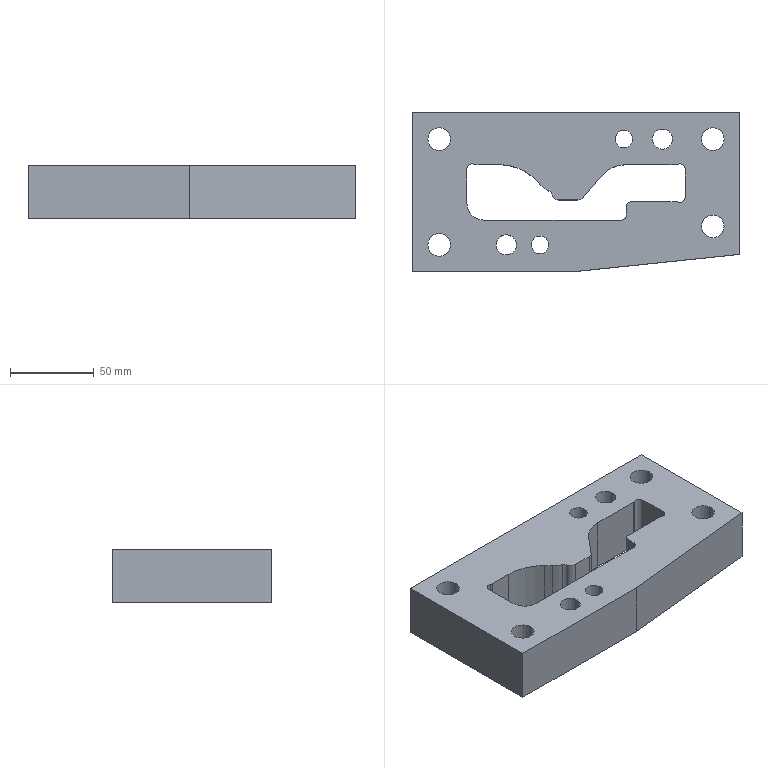Part | STEP file | lll_id254_x_t | 1 solid | 48 faces | box 195 x 95 x 32 mm | volume 434592 mm3 | cylinder 27 | plane 21 | commonest cylinder face diameters 6 x8 13.509 x4 20.008 x4 8 x3 10.505 x2 12 x2
STEP:
#1=CARTESIAN_POINT('',(479.5,-12.921,92.5));
#2=VERTEX_POINT('',#1);
#3=CARTESIAN_POINT('',(380.426,-23.25,92.5));
#4=VERTEX_POINT('',#3);
#5=CARTESIAN_POINT('',(386.882,-22.577,92.5));
#6=DIRECTION('',(-0.9946,-0.1037,0.));
#7=VECTOR('',#6,1.);
#8=LINE('',#5,#7);
#9=EDGE_CURVE('',#2,#4,#8,.T.);
#10=ORIENTED_EDGE('',*,*,#9,.F.);
#11=CARTESIAN_POINT('',(479.5,71.75,92.5));
#12=VERTEX_POINT('',#11);
#13=CARTESIAN_POINT('',(479.5,24.25,92.5));
#14=DIRECTION('',(0.,-1.,0.));
#15=VECTOR('',#14,1.);
#16=LINE('',#13,#15);
#17=EDGE_CURVE('',#12,#2,#16,.T.);
#18=ORIENTED_EDGE('',*,*,#17,.F.);
#19=CARTESIAN_POINT('',(284.5,71.75,92.5));
#20=VERTEX_POINT('',#19);
#21=CARTESIAN_POINT('',(382.,71.75,92.5));
#22=DIRECTION('',(1.,0.,0.));
#23=VECTOR('',#22,1.);
#24=LINE('',#21,#23);
#25=EDGE_CURVE('',#20,#12,#24,.T.);
#26=ORIENTED_EDGE('',*,*,#25,.F.);
#27=CARTESIAN_POINT('',(284.5,-23.25,92.5));
#28=VERTEX_POINT('',#27);
#29=CARTESIAN_POINT('',(284.5,24.25,92.5));
#30=DIRECTION('',(0.,1.,0.));
#31=VECTOR('',#30,1.);
#32=LINE('',#29,#31);
#33=EDGE_CURVE('',#28,#20,#32,.T.);
#34=ORIENTED_EDGE('',*,*,#33,.F.);
#35=CARTESIAN_POINT('',(382.,-23.25,92.5));
#36=DIRECTION('',(-1.,0.,0.));
#37=VECTOR('',#36,1.);
#38=LINE('',#35,#37);
#39=EDGE_CURVE('',#4,#28,#38,.T.);
#40=ORIENTED_EDGE('',*,*,#39,.F.);
#41=EDGE_LOOP('',(#10,#18,#26,#34,#40));
#42=FACE_BOUND('',#41,.T.);
#43=CARTESIAN_POINT('',(334.5,-7.25,92.5));
#44=VERTEX_POINT('',#43);
#45=CARTESIAN_POINT('',(340.5,-7.25,92.5));
#46=DIRECTION('',(0.,0.,1.));
#47=DIRECTION('',(-1.,0.,0.));
#48=AXIS2_PLACEMENT_3D('',#45,#46,#47);
#49=CIRCLE('',#48,6.);
#50=EDGE_CURVE('',#44,#44,#49,.T.);
#51=ORIENTED_EDGE('',*,*,#50,.F.);
#52=EDGE_LOOP('',(#51));
#53=FACE_BOUND('',#52,.T.);
#54=CARTESIAN_POINT('',(427.5,55.75,92.5));
#55=VERTEX_POINT('',#54);
#56=CARTESIAN_POINT('',(433.5,55.75,92.5));
#57=DIRECTION('',(0.,0.,1.));
#58=DIRECTION('',(-1.,0.,0.));
#59=AXIS2_PLACEMENT_3D('',#56,#57,#58);
#60=CIRCLE('',#59,6.);
#61=EDGE_CURVE('',#55,#55,#60,.T.);
#62=ORIENTED_EDGE('',*,*,#61,.F.);
#63=EDGE_LOOP('',(#62));
#64=FACE_BOUND('',#63,.T.);
#65=CARTESIAN_POINT('',(456.745,3.75,92.5));
#66=VERTEX_POINT('',#65);
#67=CARTESIAN_POINT('',(463.5,3.75,92.5));
#68=DIRECTION('',(0.,0.,1.));
#69=DIRECTION('',(-1.,0.,0.));
#70=AXIS2_PLACEMENT_3D('',#67,#68,#69);
#71=CIRCLE('',#70,6.755);
#72=EDGE_CURVE('',#66,#66,#71,.T.);
#73=ORIENTED_EDGE('',*,*,#72,.F.);
#74=EDGE_LOOP('',(#73));
#75=FACE_BOUND('',#74,.T.);
#76=CARTESIAN_POINT('',(293.745,55.75,92.5));
#77=VERTEX_POINT('',#76);
#78=CARTESIAN_POINT('',(300.5,55.75,92.5));
#79=DIRECTION('',(0.,0.,1.));
#80=DIRECTION('',(-1.,0.,0.));
#81=AXIS2_PLACEMENT_3D('',#78,#79,#80);
#82=CIRCLE('',#81,6.755);
#83=EDGE_CURVE('',#77,#77,#82,.T.);
#84=ORIENTED_EDGE('',*,*,#83,.F.);
#85=EDGE_LOOP('',(#84));
#86=FACE_BOUND('',#85,.T.);
#87=CARTESIAN_POINT('',(293.745,-7.25,92.5));
#88=VERTEX_POINT('',#87);
#89=CARTESIAN_POINT('',(300.5,-7.25,92.5));
#90=DIRECTION('',(0.,0.,1.));
#91=DIRECTION('',(-1.,0.,0.));
#92=AXIS2_PLACEMENT_3D('',#89,#90,#91);
#93=CIRCLE('',#92,6.755);
#94=EDGE_CURVE('',#88,#88,#93,.T.);
#95=ORIENTED_EDGE('',*,*,#94,.F.);
#96=EDGE_LOOP('',(#95));
#97=FACE_BOUND('',#96,.T.);
#98=CARTESIAN_POINT('',(456.745,55.75,92.5));
#99=VERTEX_POINT('',#98);
#100=CARTESIAN_POINT('',(463.5,55.75,92.5));
#101=DIRECTION('',(0.,0.,1.));
#102=DIRECTION('',(-1.,0.,0.));
#103=AXIS2_PLACEMENT_3D('',#100,#101,#102);
#104=CIRCLE('',#103,6.755);
#105=EDGE_CURVE('',#99,#99,#104,.T.);
#106=ORIENTED_EDGE('',*,*,#105,.F.);
#107=EDGE_LOOP('',(#106));
#108=FACE_BOUND('',#107,.T.);
#109=CARTESIAN_POINT('',(415.752,55.75,92.5));
#110=VERTEX_POINT('',#109);
#111=CARTESIAN_POINT('',(410.5,55.75,92.5));
#112=DIRECTION('',(0.,0.,1.));
#113=DIRECTION('',(1.,0.,0.));
#114=AXIS2_PLACEMENT_3D('',#111,#112,#113);
#115=CIRCLE('',#114,5.253);
#116=EDGE_CURVE('',#110,#110,#115,.T.);
#117=ORIENTED_EDGE('',*,*,#116,.F.);
#118=EDGE_LOOP('',(#117));
#119=FACE_BOUND('',#118,.T.);
#120=CARTESIAN_POINT('',(365.752,-7.25,92.5));
#121=VERTEX_POINT('',#120);
#122=CARTESIAN_POINT('',(360.5,-7.25,92.5));
#123=DIRECTION('',(0.,0.,1.));
#124=DIRECTION('',(1.,0.,0.));
#125=AXIS2_PLACEMENT_3D('',#122,#123,#124);
#126=CIRCLE('',#125,5.253);
#127=EDGE_CURVE('',#121,#121,#126,.T.);
#128=ORIENTED_EDGE('',*,*,#127,.F.);
#129=EDGE_LOOP('',(#128));
#130=FACE_BOUND('',#129,.T.);
#131=CARTESIAN_POINT('',(396.945,33.713,92.5));
#132=VERTEX_POINT('',#131);
#133=CARTESIAN_POINT('',(411.5,40.5,92.5));
#134=VERTEX_POINT('',#133);
#135=CARTESIAN_POINT('',(411.5,21.5,92.5));
#136=DIRECTION('',(0.,0.,-1.));
#137=DIRECTION('',(-1.,0.,0.));
#138=AXIS2_PLACEMENT_3D('',#135,#136,#137);
#139=CIRCLE('',#138,19.);
#140=EDGE_CURVE('',#132,#134,#139,.T.);
#141=ORIENTED_EDGE('',*,*,#140,.T.);
#142=CARTESIAN_POINT('',(441.602,40.5,92.5));
#143=VERTEX_POINT('',#142);
#144=CARTESIAN_POINT('',(444.,40.5,92.5));
#145=DIRECTION('',(1.,0.,0.));
#146=VECTOR('',#145,1.);
#147=LINE('',#144,#146);
#148=EDGE_CURVE('',#134,#143,#147,.T.);
#149=ORIENTED_EDGE('',*,*,#148,.T.);
#150=CARTESIAN_POINT('',(442.801,40.75,92.5));
#151=VERTEX_POINT('',#150);
#152=CARTESIAN_POINT('',(441.602,43.5,92.5));
#153=DIRECTION('',(0.,0.,1.));
#154=DIRECTION('',(-1.,0.,0.));
#155=AXIS2_PLACEMENT_3D('',#152,#153,#154);
#156=CIRCLE('',#155,3.);
#157=EDGE_CURVE('',#143,#151,#156,.T.);
#158=ORIENTED_EDGE('',*,*,#157,.T.);
#159=CARTESIAN_POINT('',(447.,38.,92.5));
#160=VERTEX_POINT('',#159);
#161=CARTESIAN_POINT('',(444.,38.,92.5));
#162=DIRECTION('',(0.,0.,-1.));
#163=DIRECTION('',(-1.,0.,0.));
#164=AXIS2_PLACEMENT_3D('',#161,#162,#163);
#165=CIRCLE('',#164,3.);
#166=EDGE_CURVE('',#151,#160,#165,.T.);
#167=ORIENTED_EDGE('',*,*,#166,.T.);
#168=CARTESIAN_POINT('',(447.,21.,92.5));
#169=VERTEX_POINT('',#168);
#170=CARTESIAN_POINT('',(447.,21.,92.5));
#171=DIRECTION('',(0.,1.,0.));
#172=VECTOR('',#171,1.);
#173=LINE('',#170,#172);
#174=EDGE_CURVE('',#169,#160,#173,.T.);
#175=ORIENTED_EDGE('',*,*,#174,.F.);
#176=CARTESIAN_POINT('',(442.801,18.25,92.5));
#177=VERTEX_POINT('',#176);
#178=CARTESIAN_POINT('',(444.,21.,92.5));
#179=DIRECTION('',(0.,0.,1.));
#180=DIRECTION('',(-1.,0.,0.));
#181=AXIS2_PLACEMENT_3D('',#178,#179,#180);
#182=CIRCLE('',#181,3.);
#183=EDGE_CURVE('',#177,#169,#182,.T.);
#184=ORIENTED_EDGE('',*,*,#183,.F.);
#185=CARTESIAN_POINT('',(441.602,18.5,92.5));
#186=VERTEX_POINT('',#185);
#187=CARTESIAN_POINT('',(441.602,15.5,92.5));
#188=DIRECTION('',(0.,0.,1.));
#189=DIRECTION('',(-1.,0.,0.));
#190=AXIS2_PLACEMENT_3D('',#187,#188,#189);
#191=CIRCLE('',#190,3.);
#192=EDGE_CURVE('',#177,#186,#191,.T.);
#193=ORIENTED_EDGE('',*,*,#192,.T.);
#194=CARTESIAN_POINT('',(415.,18.5,92.5));
#195=VERTEX_POINT('',#194);
#196=CARTESIAN_POINT('',(444.,18.5,92.5));
#197=DIRECTION('',(1.,0.,0.));
#198=VECTOR('',#197,1.);
#199=LINE('',#196,#198);
#200=EDGE_CURVE('',#195,#186,#199,.T.);
#201=ORIENTED_EDGE('',*,*,#200,.F.);
#202=CARTESIAN_POINT('',(412.,15.5,92.5));
#203=VERTEX_POINT('',#202);
#204=CARTESIAN_POINT('',(415.,15.5,92.5));
#205=DIRECTION('',(0.,0.,-1.));
#206=DIRECTION('',(-1.,0.,0.));
#207=AXIS2_PLACEMENT_3D('',#204,#205,#206);
#208=CIRCLE('',#207,3.);
#209=EDGE_CURVE('',#203,#195,#208,.T.);
#210=ORIENTED_EDGE('',*,*,#209,.F.);
#211=CARTESIAN_POINT('',(412.,10.5,92.5));
#212=VERTEX_POINT('',#211);
#213=CARTESIAN_POINT('',(412.,21.,92.5));
#214=DIRECTION('',(0.,-1.,0.));
#215=VECTOR('',#214,1.);
#216=LINE('',#213,#215);
#217=EDGE_CURVE('',#203,#212,#216,.T.);
#218=ORIENTED_EDGE('',*,*,#217,.T.);
#219=CARTESIAN_POINT('',(409.,7.5,92.5));
#220=VERTEX_POINT('',#219);
#221=CARTESIAN_POINT('',(409.,10.5,92.5));
#222=DIRECTION('',(0.,0.,-1.));
#223=DIRECTION('',(-1.,0.,0.));
#224=AXIS2_PLACEMENT_3D('',#221,#222,#223);
#225=CIRCLE('',#224,3.);
#226=EDGE_CURVE('',#212,#220,#225,.T.);
#227=ORIENTED_EDGE('',*,*,#226,.T.);
#228=CARTESIAN_POINT('',(327.,7.5,92.5));
#229=VERTEX_POINT('',#228);
#230=CARTESIAN_POINT('',(444.,7.5,92.5));
#231=DIRECTION('',(-1.,0.,0.));
#232=VECTOR('',#231,1.);
#233=LINE('',#230,#232);
#234=EDGE_CURVE('',#220,#229,#233,.T.);
#235=ORIENTED_EDGE('',*,*,#234,.T.);
#236=CARTESIAN_POINT('',(317.,17.5,92.5));
#237=VERTEX_POINT('',#236);
#238=CARTESIAN_POINT('',(327.,17.5,92.5));
#239=DIRECTION('',(0.,0.,-1.));
#240=DIRECTION('',(-1.,0.,0.));
#241=AXIS2_PLACEMENT_3D('',#238,#239,#240);
#242=CIRCLE('',#241,10.);
#243=EDGE_CURVE('',#229,#237,#242,.T.);
#244=ORIENTED_EDGE('',*,*,#243,.T.);
#245=CARTESIAN_POINT('',(317.,38.,92.5));
#246=VERTEX_POINT('',#245);
#247=CARTESIAN_POINT('',(317.,21.,92.5));
#248=DIRECTION('',(0.,-1.,0.));
#249=VECTOR('',#248,1.);
#250=LINE('',#247,#249);
#251=EDGE_CURVE('',#246,#237,#250,.T.);
#252=ORIENTED_EDGE('',*,*,#251,.F.);
#253=CARTESIAN_POINT('',(321.199,40.75,92.5));
#254=VERTEX_POINT('',#253);
#255=CARTESIAN_POINT('',(320.,38.,92.5));
#256=DIRECTION('',(0.,0.,-1.));
#257=DIRECTION('',(-1.,0.,0.));
#258=AXIS2_PLACEMENT_3D('',#255,#256,#257);
#259=CIRCLE('',#258,3.);
#260=EDGE_CURVE('',#246,#254,#259,.T.);
#261=ORIENTED_EDGE('',*,*,#260,.T.);
#262=CARTESIAN_POINT('',(322.398,40.5,92.5));
#263=VERTEX_POINT('',#262);
#264=CARTESIAN_POINT('',(322.398,43.5,92.5));
#265=DIRECTION('',(0.,0.,-1.));
#266=DIRECTION('',(-1.,0.,0.));
#267=AXIS2_PLACEMENT_3D('',#264,#265,#266);
#268=CIRCLE('',#267,3.);
#269=EDGE_CURVE('',#263,#254,#268,.T.);
#270=ORIENTED_EDGE('',*,*,#269,.F.);
#271=CARTESIAN_POINT('',(336.574,40.5,92.5));
#272=VERTEX_POINT('',#271);
#273=CARTESIAN_POINT('',(444.,40.5,92.5));
#274=DIRECTION('',(1.,0.,0.));
#275=VECTOR('',#274,1.);
#276=LINE('',#273,#275);
#277=EDGE_CURVE('',#263,#272,#276,.T.);
#278=ORIENTED_EDGE('',*,*,#277,.T.);
#279=CARTESIAN_POINT('',(357.787,31.713,92.5));
#280=VERTEX_POINT('',#279);
#281=CARTESIAN_POINT('',(336.574,10.502,92.5));
#282=DIRECTION('',(0.,0.,1.));
#283=DIRECTION('',(-1.,0.,0.));
#284=AXIS2_PLACEMENT_3D('',#281,#282,#283);
#285=CIRCLE('',#284,29.998);
#286=EDGE_CURVE('',#280,#272,#285,.T.);
#287=ORIENTED_EDGE('',*,*,#286,.F.);
#288=CARTESIAN_POINT('',(361.142,28.358,92.5));
#289=VERTEX_POINT('',#288);
#290=CARTESIAN_POINT('',(406.25,-16.75,92.5));
#291=DIRECTION('',(-0.7071,0.7071,0.));
#292=VECTOR('',#291,1.);
#293=LINE('',#290,#292);
#294=EDGE_CURVE('',#289,#280,#293,.T.);
#295=ORIENTED_EDGE('',*,*,#294,.F.);
#296=CARTESIAN_POINT('',(365.881,24.849,92.5));
#297=VERTEX_POINT('',#296);
#298=CARTESIAN_POINT('',(375.216,42.407,92.5));
#299=DIRECTION('',(0.,0.,-1.));
#300=DIRECTION('',(-1.,0.,0.));
#301=AXIS2_PLACEMENT_3D('',#298,#299,#300);
#302=CIRCLE('',#301,19.886);
#303=EDGE_CURVE('',#297,#289,#302,.T.);
#304=ORIENTED_EDGE('',*,*,#303,.F.);
#305=CARTESIAN_POINT('',(367.848,22.409,92.5));
#306=VERTEX_POINT('',#305);
#307=CARTESIAN_POINT('',(364.,21.318,92.5));
#308=DIRECTION('',(0.,0.,1.));
#309=DIRECTION('',(-1.,0.,0.));
#310=AXIS2_PLACEMENT_3D('',#307,#308,#309);
#311=CIRCLE('',#310,4.);
#312=EDGE_CURVE('',#306,#297,#311,.T.);
#313=ORIENTED_EDGE('',*,*,#312,.F.);
#314=CARTESIAN_POINT('',(371.697,19.5,92.5));
#315=VERTEX_POINT('',#314);
#316=CARTESIAN_POINT('',(371.697,23.5,92.5));
#317=DIRECTION('',(0.,0.,-1.));
#318=DIRECTION('',(-1.,0.,0.));
#319=AXIS2_PLACEMENT_3D('',#316,#317,#318);
#320=CIRCLE('',#319,4.);
#321=EDGE_CURVE('',#315,#306,#320,.T.);
#322=ORIENTED_EDGE('',*,*,#321,.F.);
#323=CARTESIAN_POINT('',(383.154,19.5,92.5));
#324=VERTEX_POINT('',#323);
#325=CARTESIAN_POINT('',(444.,19.5,92.5));
#326=DIRECTION('',(-1.,0.,0.));
#327=VECTOR('',#326,1.);
#328=LINE('',#325,#327);
#329=EDGE_CURVE('',#324,#315,#328,.T.);
#330=ORIENTED_EDGE('',*,*,#329,.F.);
#331=CARTESIAN_POINT('',(386.218,20.929,92.5));
#332=VERTEX_POINT('',#331);
#333=CARTESIAN_POINT('',(383.154,23.5,92.5));
#334=DIRECTION('',(0.,0.,1.));
#335=DIRECTION('',(-1.,0.,0.));
#336=AXIS2_PLACEMENT_3D('',#333,#334,#335);
#337=CIRCLE('',#336,4.);
#338=EDGE_CURVE('',#324,#332,#337,.T.);
#339=ORIENTED_EDGE('',*,*,#338,.T.);
#340=CARTESIAN_POINT('',(410.127,49.423,92.5));
#341=DIRECTION('',(-0.6428,-0.766,0.));
#342=VECTOR('',#341,1.);
#343=LINE('',#340,#342);
#344=EDGE_CURVE('',#132,#332,#343,.T.);
#345=ORIENTED_EDGE('',*,*,#344,.F.);
#346=EDGE_LOOP('',(#141,#149,#158,#167,#175,#184,#193,#201,#210,#218,#227,#235,#244,#252,#261,#270,#278,#287,#295,#304,#313,#322,#330,#339,#345));
#347=FACE_BOUND('',#346,.T.);
#348=CARTESIAN_POINT('',(382.,24.25,92.5));
#349=DIRECTION('',(0.,0.,1.));
#350=DIRECTION('',(-1.,0.,0.));
#351=AXIS2_PLACEMENT_3D('',#348,#349,#350);
#352=PLANE('',#351);
#353=ADVANCED_FACE('',(#42,#53,#64,#75,#86,#97,#108,#119,#130,#347),#352,.T.);
#354=CARTESIAN_POINT('',(415.752,55.75,60.5));
#355=VERTEX_POINT('',#354);
#356=CARTESIAN_POINT('',(410.5,55.75,60.5));
#357=DIRECTION('',(0.,0.,1.));
#358=DIRECTION('',(1.,0.,0.));
#359=AXIS2_PLACEMENT_3D('',#356,#357,#358);
#360=CIRCLE('',#359,5.253);
#361=EDGE_CURVE('',#355,#355,#360,.T.);
#362=ORIENTED_EDGE('',*,*,#361,.T.);
#363=EDGE_LOOP('',(#362));
#364=FACE_BOUND('',#363,.T.);
#365=CARTESIAN_POINT('',(479.5,-12.921,60.5));
#366=VERTEX_POINT('',#365);
#367=CARTESIAN_POINT('',(380.426,-23.25,60.5));
#368=VERTEX_POINT('',#367);
#369=CARTESIAN_POINT('',(479.344,-12.938,60.5));
#370=DIRECTION('',(-0.9946,-0.1037,0.));
#371=VECTOR('',#370,1.);
#372=LINE('',#369,#371);
#373=EDGE_CURVE('',#366,#368,#372,.T.);
#374=ORIENTED_EDGE('',*,*,#373,.T.);
#375=CARTESIAN_POINT('',(284.5,-23.25,60.5));
#376=VERTEX_POINT('',#375);
#377=CARTESIAN_POINT('',(382.,-23.25,60.5));
#378=DIRECTION('',(1.,0.,0.));
#379=VECTOR('',#378,1.);
#380=LINE('',#377,#379);
#381=EDGE_CURVE('',#376,#368,#380,.T.);
#382=ORIENTED_EDGE('',*,*,#381,.F.);
#383=CARTESIAN_POINT('',(284.5,71.75,60.5));
#384=VERTEX_POINT('',#383);
#385=CARTESIAN_POINT('',(284.5,24.25,60.5));
#386=DIRECTION('',(0.,-1.,0.));
#387=VECTOR('',#386,1.);
#388=LINE('',#385,#387);
#389=EDGE_CURVE('',#384,#376,#388,.T.);
#390=ORIENTED_EDGE('',*,*,#389,.F.);
#391=CARTESIAN_POINT('',(479.5,71.75,60.5));
#392=VERTEX_POINT('',#391);
#393=CARTESIAN_POINT('',(382.,71.75,60.5));
#394=DIRECTION('',(-1.,0.,0.));
#395=VECTOR('',#394,1.);
#396=LINE('',#393,#395);
#397=EDGE_CURVE('',#392,#384,#396,.T.);
#398=ORIENTED_EDGE('',*,*,#397,.F.);
#399=CARTESIAN_POINT('',(479.5,24.25,60.5));
#400=DIRECTION('',(0.,1.,0.));
#401=VECTOR('',#400,1.);
#402=LINE('',#399,#401);
#403=EDGE_CURVE('',#366,#392,#402,.T.);
#404=ORIENTED_EDGE('',*,*,#403,.F.);
#405=EDGE_LOOP('',(#374,#382,#390,#398,#404));
#406=FACE_BOUND('',#405,.T.);
#407=CARTESIAN_POINT('',(346.5,-7.25,60.5));
#408=VERTEX_POINT('',#407);
#409=CARTESIAN_POINT('',(340.5,-7.25,60.5));
#410=DIRECTION('',(0.,0.,-1.));
#411=DIRECTION('',(1.,0.,0.));
#412=AXIS2_PLACEMENT_3D('',#409,#410,#411);
#413=CIRCLE('',#412,6.);
#414=EDGE_CURVE('',#408,#408,#413,.T.);
#415=ORIENTED_EDGE('',*,*,#414,.F.);
#416=EDGE_LOOP('',(#415));
#417=FACE_BOUND('',#416,.T.);
#418=CARTESIAN_POINT('',(439.5,55.75,60.5));
#419=VERTEX_POINT('',#418);
#420=CARTESIAN_POINT('',(433.5,55.75,60.5));
#421=DIRECTION('',(0.,0.,-1.));
#422=DIRECTION('',(1.,0.,0.));
#423=AXIS2_PLACEMENT_3D('',#420,#421,#422);
#424=CIRCLE('',#423,6.);
#425=EDGE_CURVE('',#419,#419,#424,.T.);
#426=ORIENTED_EDGE('',*,*,#425,.F.);
#427=EDGE_LOOP('',(#426));
#428=FACE_BOUND('',#427,.T.);
#429=CARTESIAN_POINT('',(290.496,55.75,60.5));
#430=VERTEX_POINT('',#429);
#431=CARTESIAN_POINT('',(300.5,55.75,60.5));
#432=DIRECTION('',(0.,0.,1.));
#433=DIRECTION('',(-1.,0.,0.));
#434=AXIS2_PLACEMENT_3D('',#431,#432,#433);
#435=CIRCLE('',#434,10.004);
#436=EDGE_CURVE('',#430,#430,#435,.T.);
#437=ORIENTED_EDGE('',*,*,#436,.T.);
#438=EDGE_LOOP('',(#437));
#439=FACE_BOUND('',#438,.T.);
#440=CARTESIAN_POINT('',(453.496,55.75,60.5));
#441=VERTEX_POINT('',#440);
#442=CARTESIAN_POINT('',(463.5,55.75,60.5));
#443=DIRECTION('',(0.,0.,1.));
#444=DIRECTION('',(-1.,0.,0.));
#445=AXIS2_PLACEMENT_3D('',#442,#443,#444);
#446=CIRCLE('',#445,10.004);
#447=EDGE_CURVE('',#441,#441,#446,.T.);
#448=ORIENTED_EDGE('',*,*,#447,.T.);
#449=EDGE_LOOP('',(#448));
#450=FACE_BOUND('',#449,.T.);
#451=CARTESIAN_POINT('',(290.496,-7.25,60.5));
#452=VERTEX_POINT('',#451);
#453=CARTESIAN_POINT('',(300.5,-7.25,60.5));
#454=DIRECTION('',(0.,0.,1.));
#455=DIRECTION('',(-1.,0.,0.));
#456=AXIS2_PLACEMENT_3D('',#453,#454,#455);
#457=CIRCLE('',#456,10.004);
#458=EDGE_CURVE('',#452,#452,#457,.T.);
#459=ORIENTED_EDGE('',*,*,#458,.T.);
#460=EDGE_LOOP('',(#459));
#461=FACE_BOUND('',#460,.T.);
#462=CARTESIAN_POINT('',(453.496,3.75,60.5));
#463=VERTEX_POINT('',#462);
#464=CARTESIAN_POINT('',(463.5,3.75,60.5));
#465=DIRECTION('',(0.,0.,1.));
#466=DIRECTION('',(-1.,0.,0.));
#467=AXIS2_PLACEMENT_3D('',#464,#465,#466);
#468=CIRCLE('',#467,10.004);
#469=EDGE_CURVE('',#463,#463,#468,.T.);
#470=ORIENTED_EDGE('',*,*,#469,.T.);
#471=EDGE_LOOP('',(#470));
#472=FACE_BOUND('',#471,.T.);
#473=CARTESIAN_POINT('',(365.752,-7.25,60.5));
#474=VERTEX_POINT('',#473);
#475=CARTESIAN_POINT('',(360.5,-7.25,60.5));
#476=DIRECTION('',(0.,0.,1.));
#477=DIRECTION('',(1.,0.,0.));
#478=AXIS2_PLACEMENT_3D('',#475,#476,#477);
#479=CIRCLE('',#478,5.253);
#480=EDGE_CURVE('',#474,#474,#479,.T.);
#481=ORIENTED_EDGE('',*,*,#480,.T.);
#482=EDGE_LOOP('',(#481));
#483=FACE_BOUND('',#482,.T.);
#484=CARTESIAN_POINT('',(441.602,40.5,60.5));
#485=VERTEX_POINT('',#484);
#486=CARTESIAN_POINT('',(411.5,40.5,60.5));
#487=VERTEX_POINT('',#486);
#488=CARTESIAN_POINT('',(441.602,40.5,60.5));
#489=DIRECTION('',(-1.,0.,0.));
#490=VECTOR('',#489,1.);
#491=LINE('',#488,#490);
#492=EDGE_CURVE('',#485,#487,#491,.T.);
#493=ORIENTED_EDGE('',*,*,#492,.T.);
#494=CARTESIAN_POINT('',(396.945,33.713,60.5));
#495=VERTEX_POINT('',#494);
#496=CARTESIAN_POINT('',(411.5,21.5,60.5));
#497=DIRECTION('',(0.,0.,-1.));
#498=DIRECTION('',(-1.,0.,0.));
#499=AXIS2_PLACEMENT_3D('',#496,#497,#498);
#500=CIRCLE('',#499,19.);
#501=EDGE_CURVE('',#495,#487,#500,.T.);
#502=ORIENTED_EDGE('',*,*,#501,.F.);
#503=CARTESIAN_POINT('',(386.218,20.929,60.5));
#504=VERTEX_POINT('',#503);
#505=CARTESIAN_POINT('',(396.945,33.713,60.5));
#506=DIRECTION('',(-0.6428,-0.766,0.));
#507=VECTOR('',#506,1.);
#508=LINE('',#505,#507);
#509=EDGE_CURVE('',#495,#504,#508,.T.);
#510=ORIENTED_EDGE('',*,*,#509,.T.);
#511=CARTESIAN_POINT('',(383.154,19.5,60.5));
#512=VERTEX_POINT('',#511);
#513=CARTESIAN_POINT('',(383.154,23.5,60.5));
#514=DIRECTION('',(0.,0.,1.));
#515=DIRECTION('',(-1.,0.,0.));
#516=AXIS2_PLACEMENT_3D('',#513,#514,#515);
#517=CIRCLE('',#516,4.);
#518=EDGE_CURVE('',#512,#504,#517,.T.);
#519=ORIENTED_EDGE('',*,*,#518,.F.);
#520=CARTESIAN_POINT('',(371.697,19.5,60.5));
#521=VERTEX_POINT('',#520);
#522=CARTESIAN_POINT('',(383.154,19.5,60.5));
#523=DIRECTION('',(-1.,0.,0.));
#524=VECTOR('',#523,1.);
#525=LINE('',#522,#524);
#526=EDGE_CURVE('',#512,#521,#525,.T.);
#527=ORIENTED_EDGE('',*,*,#526,.T.);
#528=CARTESIAN_POINT('',(367.848,22.409,60.5));
#529=VERTEX_POINT('',#528);
#530=CARTESIAN_POINT('',(371.697,23.5,60.5));
#531=DIRECTION('',(0.,0.,-1.));
#532=DIRECTION('',(-1.,0.,0.));
#533=AXIS2_PLACEMENT_3D('',#530,#531,#532);
#534=CIRCLE('',#533,4.);
#535=EDGE_CURVE('',#521,#529,#534,.T.);
#536=ORIENTED_EDGE('',*,*,#535,.T.);
#537=CARTESIAN_POINT('',(365.881,24.849,60.5));
#538=VERTEX_POINT('',#537);
#539=CARTESIAN_POINT('',(364.,21.318,60.5));
#540=DIRECTION('',(0.,0.,1.));
#541=DIRECTION('',(-1.,0.,0.));
#542=AXIS2_PLACEMENT_3D('',#539,#540,#541);
#543=CIRCLE('',#542,4.);
#544=EDGE_CURVE('',#529,#538,#543,.T.);
#545=ORIENTED_EDGE('',*,*,#544,.T.);
#546=CARTESIAN_POINT('',(361.142,28.358,60.5));
#547=VERTEX_POINT('',#546);
#548=CARTESIAN_POINT('',(375.216,42.407,60.5));
#549=DIRECTION('',(0.,0.,-1.));
#550=DIRECTION('',(-1.,0.,0.));
#551=AXIS2_PLACEMENT_3D('',#548,#549,#550);
#552=CIRCLE('',#551,19.886);
#553=EDGE_CURVE('',#538,#547,#552,.T.);
#554=ORIENTED_EDGE('',*,*,#553,.T.);
#555=CARTESIAN_POINT('',(357.787,31.713,60.5));
#556=VERTEX_POINT('',#555);
#557=CARTESIAN_POINT('',(361.142,28.358,60.5));
#558=DIRECTION('',(-0.7071,0.7071,0.));
#559=VECTOR('',#558,1.);
#560=LINE('',#557,#559);
#561=EDGE_CURVE('',#547,#556,#560,.T.);
#562=ORIENTED_EDGE('',*,*,#561,.T.);
#563=CARTESIAN_POINT('',(336.574,40.5,60.5));
#564=VERTEX_POINT('',#563);
#565=CARTESIAN_POINT('',(336.574,10.502,60.5));
#566=DIRECTION('',(0.,0.,-1.));
#567=DIRECTION('',(-1.,0.,0.));
#568=AXIS2_PLACEMENT_3D('',#565,#566,#567);
#569=CIRCLE('',#568,29.998);
#570=EDGE_CURVE('',#564,#556,#569,.T.);
#571=ORIENTED_EDGE('',*,*,#570,.F.);
#572=CARTESIAN_POINT('',(322.398,40.5,60.5));
#573=VERTEX_POINT('',#572);
#574=CARTESIAN_POINT('',(336.574,40.5,60.5));
#575=DIRECTION('',(1.,0.,0.));
#576=VECTOR('',#575,1.);
#577=LINE('',#574,#576);
#578=EDGE_CURVE('',#573,#564,#577,.T.);
#579=ORIENTED_EDGE('',*,*,#578,.F.);
#580=CARTESIAN_POINT('',(321.199,40.75,60.5));
#581=VERTEX_POINT('',#580);
#582=CARTESIAN_POINT('',(322.398,43.5,60.5));
#583=DIRECTION('',(0.,0.,-1.));
#584=DIRECTION('',(-1.,0.,0.));
#585=AXIS2_PLACEMENT_3D('',#582,#583,#584);
#586=CIRCLE('',#585,3.);
#587=EDGE_CURVE('',#573,#581,#586,.T.);
#588=ORIENTED_EDGE('',*,*,#587,.T.);
#589=CARTESIAN_POINT('',(317.,38.,60.5));
#590=VERTEX_POINT('',#589);
#591=CARTESIAN_POINT('',(320.,38.,60.5));
#592=DIRECTION('',(0.,0.,1.));
#593=DIRECTION('',(-1.,0.,0.));
#594=AXIS2_PLACEMENT_3D('',#591,#592,#593);
#595=CIRCLE('',#594,3.);
#596=EDGE_CURVE('',#581,#590,#595,.T.);
#597=ORIENTED_EDGE('',*,*,#596,.T.);
#598=CARTESIAN_POINT('',(317.,17.5,60.5));
#599=VERTEX_POINT('',#598);
#600=CARTESIAN_POINT('',(317.,38.,60.5));
#601=DIRECTION('',(0.,-1.,0.));
#602=VECTOR('',#601,1.);
#603=LINE('',#600,#602);
#604=EDGE_CURVE('',#590,#599,#603,.T.);
#605=ORIENTED_EDGE('',*,*,#604,.T.);
#606=CARTESIAN_POINT('',(327.,7.5,60.5));
#607=VERTEX_POINT('',#606);
#608=CARTESIAN_POINT('',(327.,17.5,60.5));
#609=DIRECTION('',(0.,0.,1.));
#610=DIRECTION('',(-1.,0.,0.));
#611=AXIS2_PLACEMENT_3D('',#608,#609,#610);
#612=CIRCLE('',#611,10.);
#613=EDGE_CURVE('',#599,#607,#612,.T.);
#614=ORIENTED_EDGE('',*,*,#613,.T.);
#615=CARTESIAN_POINT('',(409.,7.5,60.5));
#616=VERTEX_POINT('',#615);
#617=CARTESIAN_POINT('',(327.,7.5,60.5));
#618=DIRECTION('',(-1.,0.,0.));
#619=VECTOR('',#618,1.);
#620=LINE('',#617,#619);
#621=EDGE_CURVE('',#616,#607,#620,.T.);
#622=ORIENTED_EDGE('',*,*,#621,.F.);
#623=CARTESIAN_POINT('',(412.,10.5,60.5));
#624=VERTEX_POINT('',#623);
#625=CARTESIAN_POINT('',(409.,10.5,60.5));
#626=DIRECTION('',(0.,0.,-1.));
#627=DIRECTION('',(-1.,0.,0.));
#628=AXIS2_PLACEMENT_3D('',#625,#626,#627);
#629=CIRCLE('',#628,3.);
#630=EDGE_CURVE('',#624,#616,#629,.T.);
#631=ORIENTED_EDGE('',*,*,#630,.F.);
#632=CARTESIAN_POINT('',(412.,15.5,60.5));
#633=VERTEX_POINT('',#632);
#634=CARTESIAN_POINT('',(412.,10.5,60.5));
#635=DIRECTION('',(0.,-1.,0.));
#636=VECTOR('',#635,1.);
#637=LINE('',#634,#636);
#638=EDGE_CURVE('',#633,#624,#637,.T.);
#639=ORIENTED_EDGE('',*,*,#638,.F.);
#640=CARTESIAN_POINT('',(415.,18.5,60.5));
#641=VERTEX_POINT('',#640);
#642=CARTESIAN_POINT('',(415.,15.5,60.5));
#643=DIRECTION('',(0.,0.,1.));
#644=DIRECTION('',(-1.,0.,0.));
#645=AXIS2_PLACEMENT_3D('',#642,#643,#644);
#646=CIRCLE('',#645,3.);
#647=EDGE_CURVE('',#641,#633,#646,.T.);
#648=ORIENTED_EDGE('',*,*,#647,.F.);
#649=CARTESIAN_POINT('',(441.602,18.5,60.5));
#650=VERTEX_POINT('',#649);
#651=CARTESIAN_POINT('',(415.,18.5,60.5));
#652=DIRECTION('',(-1.,0.,0.));
#653=VECTOR('',#652,1.);
#654=LINE('',#651,#653);
#655=EDGE_CURVE('',#650,#641,#654,.T.);
#656=ORIENTED_EDGE('',*,*,#655,.F.);
#657=CARTESIAN_POINT('',(442.801,18.25,60.5));
#658=VERTEX_POINT('',#657);
#659=CARTESIAN_POINT('',(441.602,15.5,60.5));
#660=DIRECTION('',(0.,0.,1.));
#661=DIRECTION('',(-1.,0.,0.));
#662=AXIS2_PLACEMENT_3D('',#659,#660,#661);
#663=CIRCLE('',#662,3.);
#664=EDGE_CURVE('',#658,#650,#663,.T.);
#665=ORIENTED_EDGE('',*,*,#664,.F.);
#666=CARTESIAN_POINT('',(447.,21.,60.5));
#667=VERTEX_POINT('',#666);
#668=CARTESIAN_POINT('',(444.,21.,60.5));
#669=DIRECTION('',(0.,0.,1.));
#670=DIRECTION('',(-1.,0.,0.));
#671=AXIS2_PLACEMENT_3D('',#668,#669,#670);
#672=CIRCLE('',#671,3.);
#673=EDGE_CURVE('',#658,#667,#672,.T.);
#674=ORIENTED_EDGE('',*,*,#673,.T.);
#675=CARTESIAN_POINT('',(447.,38.,60.5));
#676=VERTEX_POINT('',#675);
#677=CARTESIAN_POINT('',(447.,21.,60.5));
#678=DIRECTION('',(0.,-1.,0.));
#679=VECTOR('',#678,1.);
#680=LINE('',#677,#679);
#681=EDGE_CURVE('',#676,#667,#680,.T.);
#682=ORIENTED_EDGE('',*,*,#681,.F.);
#683=CARTESIAN_POINT('',(442.801,40.75,60.5));
#684=VERTEX_POINT('',#683);
#685=CARTESIAN_POINT('',(444.,38.,60.5));
#686=DIRECTION('',(0.,0.,-1.));
#687=DIRECTION('',(-1.,0.,0.));
#688=AXIS2_PLACEMENT_3D('',#685,#686,#687);
#689=CIRCLE('',#688,3.);
#690=EDGE_CURVE('',#684,#676,#689,.T.);
#691=ORIENTED_EDGE('',*,*,#690,.F.);
#692=CARTESIAN_POINT('',(441.602,43.5,60.5));
#693=DIRECTION('',(0.,0.,1.));
#694=DIRECTION('',(-1.,0.,0.));
#695=AXIS2_PLACEMENT_3D('',#692,#693,#694);
#696=CIRCLE('',#695,3.);
#697=EDGE_CURVE('',#485,#684,#696,.T.);
#698=ORIENTED_EDGE('',*,*,#697,.F.);
#699=EDGE_LOOP('',(#493,#502,#510,#519,#527,#536,#545,#554,#562,#571,#579,#588,#597,#605,#614,#622,#631,#639,#648,#656,#665,#674,#682,#691,#698));
#700=FACE_BOUND('',#699,.T.);
#701=CARTESIAN_POINT('',(382.,24.25,60.5));
#702=DIRECTION('',(0.,0.,-1.));
#703=DIRECTION('',(1.,0.,0.));
#704=AXIS2_PLACEMENT_3D('',#701,#702,#703);
#705=PLANE('',#704);
#706=ADVANCED_FACE('',(#364,#406,#417,#428,#439,#450,#461,#472,#483,#700),#705,.T.);
#707=CARTESIAN_POINT('',(284.5,71.75,60.5));
#708=DIRECTION('',(0.,0.,1.));
#709=VECTOR('',#708,1.);
#710=LINE('',#707,#709);
#711=EDGE_CURVE('',#384,#20,#710,.T.);
#712=ORIENTED_EDGE('',*,*,#711,.T.);
#713=ORIENTED_EDGE('',*,*,#25,.T.);
#714=CARTESIAN_POINT('',(479.5,71.75,60.5));
#715=DIRECTION('',(0.,0.,1.));
#716=VECTOR('',#715,1.);
#717=LINE('',#714,#716);
#718=EDGE_CURVE('',#392,#12,#717,.T.);
#719=ORIENTED_EDGE('',*,*,#718,.F.);
#720=ORIENTED_EDGE('',*,*,#397,.T.);
#721=EDGE_LOOP('',(#712,#713,#719,#720));
#722=FACE_OUTER_BOUND('',#721,.T.);
#723=CARTESIAN_POINT('',(382.,71.75,60.5));
#724=DIRECTION('',(0.,1.,0.));
#725=DIRECTION('',(0.,0.,-1.));
#726=AXIS2_PLACEMENT_3D('',#723,#724,#725);
#727=PLANE('',#726);
#728=ADVANCED_FACE('',(#722),#727,.T.);
#729=CARTESIAN_POINT('',(479.5,-12.921,60.5));
#730=DIRECTION('',(0.,0.,1.));
#731=VECTOR('',#730,1.);
#732=LINE('',#729,#731);
#733=EDGE_CURVE('',#366,#2,#732,.T.);
#734=ORIENTED_EDGE('',*,*,#733,.F.);
#735=ORIENTED_EDGE('',*,*,#403,.T.);
#736=ORIENTED_EDGE('',*,*,#718,.T.);
#737=ORIENTED_EDGE('',*,*,#17,.T.);
#738=EDGE_LOOP('',(#734,#735,#736,#737));
#739=FACE_OUTER_BOUND('',#738,.T.);
#740=CARTESIAN_POINT('',(479.5,24.25,60.5));
#741=DIRECTION('',(1.,0.,0.));
#742=DIRECTION('',(0.,0.,1.));
#743=AXIS2_PLACEMENT_3D('',#740,#741,#742);
#744=PLANE('',#743);
#745=ADVANCED_FACE('',(#739),#744,.T.);
#746=CARTESIAN_POINT('',(380.426,-23.25,60.5));
#747=DIRECTION('',(0.,0.,-1.));
#748=VECTOR('',#747,1.);
#749=LINE('',#746,#748);
#750=EDGE_CURVE('',#4,#368,#749,.T.);
#751=ORIENTED_EDGE('',*,*,#750,.F.);
#752=ORIENTED_EDGE('',*,*,#39,.T.);
#753=CARTESIAN_POINT('',(284.5,-23.25,60.5));
#754=DIRECTION('',(0.,0.,1.));
#755=VECTOR('',#754,1.);
#756=LINE('',#753,#755);
#757=EDGE_CURVE('',#376,#28,#756,.T.);
#758=ORIENTED_EDGE('',*,*,#757,.F.);
#759=ORIENTED_EDGE('',*,*,#381,.T.);
#760=EDGE_LOOP('',(#751,#752,#758,#759));
#761=FACE_OUTER_BOUND('',#760,.T.);
#762=CARTESIAN_POINT('',(382.,-23.25,60.5));
#763=DIRECTION('',(0.,-1.,0.));
#764=DIRECTION('',(0.,0.,1.));
#765=AXIS2_PLACEMENT_3D('',#762,#763,#764);
#766=PLANE('',#765);
#767=ADVANCED_FACE('',(#761),#766,.T.);
#768=ORIENTED_EDGE('',*,*,#389,.T.);
#769=ORIENTED_EDGE('',*,*,#757,.T.);
#770=ORIENTED_EDGE('',*,*,#33,.T.);
#771=ORIENTED_EDGE('',*,*,#711,.F.);
#772=EDGE_LOOP('',(#768,#769,#770,#771));
#773=FACE_OUTER_BOUND('',#772,.T.);
#774=CARTESIAN_POINT('',(284.5,24.25,60.5));
#775=DIRECTION('',(-1.,0.,0.));
#776=DIRECTION('',(0.,0.,-1.));
#777=AXIS2_PLACEMENT_3D('',#774,#775,#776);
#778=PLANE('',#777);
#779=ADVANCED_FACE('',(#773),#778,.T.);
#780=ORIENTED_EDGE('',*,*,#105,.T.);
#781=EDGE_LOOP('',(#780));
#782=FACE_BOUND('',#781,.T.);
#783=CARTESIAN_POINT('',(456.745,55.75,75.5));
#784=VERTEX_POINT('',#783);
#785=CARTESIAN_POINT('',(463.5,55.75,75.5));
#786=DIRECTION('',(0.,0.,1.));
#787=DIRECTION('',(-1.,0.,0.));
#788=AXIS2_PLACEMENT_3D('',#785,#786,#787);
#789=CIRCLE('',#788,6.755);
#790=EDGE_CURVE('',#784,#784,#789,.T.);
#791=ORIENTED_EDGE('',*,*,#790,.F.);
#792=EDGE_LOOP('',(#791));
#793=FACE_BOUND('',#792,.T.);
#794=CARTESIAN_POINT('',(463.5,55.75,57.5));
#795=DIRECTION('',(0.,0.,1.));
#796=DIRECTION('',(-1.,0.,0.));
#797=AXIS2_PLACEMENT_3D('',#794,#795,#796);
#798=CYLINDRICAL_SURFACE('',#797,6.755);
#799=ADVANCED_FACE('',(#782,#793),#798,.F.);
#800=ORIENTED_EDGE('',*,*,#790,.T.);
#801=EDGE_LOOP('',(#800));
#802=FACE_BOUND('',#801,.T.);
#803=CARTESIAN_POINT('',(453.496,55.75,75.5));
#804=VERTEX_POINT('',#803);
#805=CARTESIAN_POINT('',(463.5,55.75,75.5));
#806=DIRECTION('',(0.,0.,1.));
#807=DIRECTION('',(-1.,0.,0.));
#808=AXIS2_PLACEMENT_3D('',#805,#806,#807);
#809=CIRCLE('',#808,10.004);
#810=EDGE_CURVE('',#804,#804,#809,.T.);
#811=ORIENTED_EDGE('',*,*,#810,.F.);
#812=EDGE_LOOP('',(#811));
#813=FACE_BOUND('',#812,.T.);
#814=CARTESIAN_POINT('',(463.5,55.75,75.5));
#815=DIRECTION('',(0.,0.,1.));
#816=DIRECTION('',(-1.,0.,0.));
#817=AXIS2_PLACEMENT_3D('',#814,#815,#816);
#818=PLANE('',#817);
#819=ADVANCED_FACE('',(#802,#813),#818,.F.);
#820=ORIENTED_EDGE('',*,*,#810,.T.);
#821=EDGE_LOOP('',(#820));
#822=FACE_BOUND('',#821,.T.);
#823=ORIENTED_EDGE('',*,*,#447,.F.);
#824=EDGE_LOOP('',(#823));
#825=FACE_BOUND('',#824,.T.);
#826=CARTESIAN_POINT('',(463.5,55.75,60.5));
#827=DIRECTION('',(0.,0.,1.));
#828=DIRECTION('',(-1.,0.,0.));
#829=AXIS2_PLACEMENT_3D('',#826,#827,#828);
#830=CYLINDRICAL_SURFACE('',#829,10.004);
#831=ADVANCED_FACE('',(#822,#825),#830,.F.);
#832=ORIENTED_EDGE('',*,*,#94,.T.);
#833=EDGE_LOOP('',(#832));
#834=FACE_BOUND('',#833,.T.);
#835=CARTESIAN_POINT('',(293.745,-7.25,75.5));
#836=VERTEX_POINT('',#835);
#837=CARTESIAN_POINT('',(300.5,-7.25,75.5));
#838=DIRECTION('',(0.,0.,1.));
#839=DIRECTION('',(-1.,0.,0.));
#840=AXIS2_PLACEMENT_3D('',#837,#838,#839);
#841=CIRCLE('',#840,6.755);
#842=EDGE_CURVE('',#836,#836,#841,.T.);
#843=ORIENTED_EDGE('',*,*,#842,.F.);
#844=EDGE_LOOP('',(#843));
#845=FACE_BOUND('',#844,.T.);
#846=CARTESIAN_POINT('',(300.5,-7.25,57.5));
#847=DIRECTION('',(0.,0.,1.));
#848=DIRECTION('',(-1.,0.,0.));
#849=AXIS2_PLACEMENT_3D('',#846,#847,#848);
#850=CYLINDRICAL_SURFACE('',#849,6.755);
#851=ADVANCED_FACE('',(#834,#845),#850,.F.);
#852=ORIENTED_EDGE('',*,*,#842,.T.);
#853=EDGE_LOOP('',(#852));
#854=FACE_BOUND('',#853,.T.);
#855=CARTESIAN_POINT('',(290.496,-7.25,75.5));
#856=VERTEX_POINT('',#855);
#857=CARTESIAN_POINT('',(300.5,-7.25,75.5));
#858=DIRECTION('',(0.,0.,1.));
#859=DIRECTION('',(-1.,0.,0.));
#860=AXIS2_PLACEMENT_3D('',#857,#858,#859);
#861=CIRCLE('',#860,10.004);
#862=EDGE_CURVE('',#856,#856,#861,.T.);
#863=ORIENTED_EDGE('',*,*,#862,.F.);
#864=EDGE_LOOP('',(#863));
#865=FACE_BOUND('',#864,.T.);
#866=CARTESIAN_POINT('',(300.5,-7.25,75.5));
#867=DIRECTION('',(0.,0.,1.));
#868=DIRECTION('',(-1.,0.,0.));
#869=AXIS2_PLACEMENT_3D('',#866,#867,#868);
#870=PLANE('',#869);
#871=ADVANCED_FACE('',(#854,#865),#870,.F.);
#872=ORIENTED_EDGE('',*,*,#862,.T.);
#873=EDGE_LOOP('',(#872));
#874=FACE_BOUND('',#873,.T.);
#875=ORIENTED_EDGE('',*,*,#458,.F.);
#876=EDGE_LOOP('',(#875));
#877=FACE_BOUND('',#876,.T.);
#878=CARTESIAN_POINT('',(300.5,-7.25,60.5));
#879=DIRECTION('',(0.,0.,1.));
#880=DIRECTION('',(-1.,0.,0.));
#881=AXIS2_PLACEMENT_3D('',#878,#879,#880);
#882=CYLINDRICAL_SURFACE('',#881,10.004);
#883=ADVANCED_FACE('',(#874,#877),#882,.F.);
#884=ORIENTED_EDGE('',*,*,#83,.T.);
#885=EDGE_LOOP('',(#884));
#886=FACE_BOUND('',#885,.T.);
#887=CARTESIAN_POINT('',(293.745,55.75,75.5));
#888=VERTEX_POINT('',#887);
#889=CARTESIAN_POINT('',(300.5,55.75,75.5));
#890=DIRECTION('',(0.,0.,1.));
#891=DIRECTION('',(-1.,0.,0.));
#892=AXIS2_PLACEMENT_3D('',#889,#890,#891);
#893=CIRCLE('',#892,6.755);
#894=EDGE_CURVE('',#888,#888,#893,.T.);
#895=ORIENTED_EDGE('',*,*,#894,.F.);
#896=EDGE_LOOP('',(#895));
#897=FACE_BOUND('',#896,.T.);
#898=CARTESIAN_POINT('',(300.5,55.75,57.5));
#899=DIRECTION('',(0.,0.,1.));
#900=DIRECTION('',(-1.,0.,0.));
#901=AXIS2_PLACEMENT_3D('',#898,#899,#900);
#902=CYLINDRICAL_SURFACE('',#901,6.755);
#903=ADVANCED_FACE('',(#886,#897),#902,.F.);
#904=ORIENTED_EDGE('',*,*,#894,.T.);
#905=EDGE_LOOP('',(#904));
#906=FACE_BOUND('',#905,.T.);
#907=CARTESIAN_POINT('',(290.496,55.75,75.5));
#908=VERTEX_POINT('',#907);
#909=CARTESIAN_POINT('',(300.5,55.75,75.5));
#910=DIRECTION('',(0.,0.,1.));
#911=DIRECTION('',(-1.,0.,0.));
#912=AXIS2_PLACEMENT_3D('',#909,#910,#911);
#913=CIRCLE('',#912,10.004);
#914=EDGE_CURVE('',#908,#908,#913,.T.);
#915=ORIENTED_EDGE('',*,*,#914,.F.);
#916=EDGE_LOOP('',(#915));
#917=FACE_BOUND('',#916,.T.);
#918=CARTESIAN_POINT('',(300.5,55.75,75.5));
#919=DIRECTION('',(0.,0.,1.));
#920=DIRECTION('',(-1.,0.,0.));
#921=AXIS2_PLACEMENT_3D('',#918,#919,#920);
#922=PLANE('',#921);
#923=ADVANCED_FACE('',(#906,#917),#922,.F.);
#924=ORIENTED_EDGE('',*,*,#914,.T.);
#925=EDGE_LOOP('',(#924));
#926=FACE_BOUND('',#925,.T.);
#927=ORIENTED_EDGE('',*,*,#436,.F.);
#928=EDGE_LOOP('',(#927));
#929=FACE_BOUND('',#928,.T.);
#930=CARTESIAN_POINT('',(300.5,55.75,60.5));
#931=DIRECTION('',(0.,0.,1.));
#932=DIRECTION('',(-1.,0.,0.));
#933=AXIS2_PLACEMENT_3D('',#930,#931,#932);
#934=CYLINDRICAL_SURFACE('',#933,10.004);
#935=ADVANCED_FACE('',(#926,#929),#934,.F.);
#936=ORIENTED_EDGE('',*,*,#72,.T.);
#937=EDGE_LOOP('',(#936));
#938=FACE_BOUND('',#937,.T.);
#939=CARTESIAN_POINT('',(456.745,3.75,75.5));
#940=VERTEX_POINT('',#939);
#941=CARTESIAN_POINT('',(463.5,3.75,75.5));
#942=DIRECTION('',(0.,0.,1.));
#943=DIRECTION('',(-1.,0.,0.));
#944=AXIS2_PLACEMENT_3D('',#941,#942,#943);
#945=CIRCLE('',#944,6.755);
#946=EDGE_CURVE('',#940,#940,#945,.T.);
#947=ORIENTED_EDGE('',*,*,#946,.F.);
#948=EDGE_LOOP('',(#947));
#949=FACE_BOUND('',#948,.T.);
#950=CARTESIAN_POINT('',(463.5,3.75,57.5));
#951=DIRECTION('',(0.,0.,1.));
#952=DIRECTION('',(-1.,0.,0.));
#953=AXIS2_PLACEMENT_3D('',#950,#951,#952);
#954=CYLINDRICAL_SURFACE('',#953,6.755);
#955=ADVANCED_FACE('',(#938,#949),#954,.F.);
#956=ORIENTED_EDGE('',*,*,#946,.T.);
#957=EDGE_LOOP('',(#956));
#958=FACE_BOUND('',#957,.T.);
#959=CARTESIAN_POINT('',(453.496,3.75,75.5));
#960=VERTEX_POINT('',#959);
#961=CARTESIAN_POINT('',(463.5,3.75,75.5));
#962=DIRECTION('',(0.,0.,1.));
#963=DIRECTION('',(-1.,0.,0.));
#964=AXIS2_PLACEMENT_3D('',#961,#962,#963);
#965=CIRCLE('',#964,10.004);
#966=EDGE_CURVE('',#960,#960,#965,.T.);
#967=ORIENTED_EDGE('',*,*,#966,.F.);
#968=EDGE_LOOP('',(#967));
#969=FACE_BOUND('',#968,.T.);
#970=CARTESIAN_POINT('',(463.5,3.75,75.5));
#971=DIRECTION('',(0.,0.,1.));
#972=DIRECTION('',(-1.,0.,0.));
#973=AXIS2_PLACEMENT_3D('',#970,#971,#972);
#974=PLANE('',#973);
#975=ADVANCED_FACE('',(#958,#969),#974,.F.);
#976=ORIENTED_EDGE('',*,*,#966,.T.);
#977=EDGE_LOOP('',(#976));
#978=FACE_BOUND('',#977,.T.);
#979=ORIENTED_EDGE('',*,*,#469,.F.);
#980=EDGE_LOOP('',(#979));
#981=FACE_BOUND('',#980,.T.);
#982=CARTESIAN_POINT('',(463.5,3.75,60.5));
#983=DIRECTION('',(0.,0.,1.));
#984=DIRECTION('',(-1.,0.,0.));
#985=AXIS2_PLACEMENT_3D('',#982,#983,#984);
#986=CYLINDRICAL_SURFACE('',#985,10.004);
#987=ADVANCED_FACE('',(#978,#981),#986,.F.);
#988=ORIENTED_EDGE('',*,*,#425,.T.);
#989=EDGE_LOOP('',(#988));
#990=FACE_BOUND('',#989,.T.);
#991=ORIENTED_EDGE('',*,*,#61,.T.);
#992=EDGE_LOOP('',(#991));
#993=FACE_BOUND('',#992,.T.);
#994=CARTESIAN_POINT('',(433.5,55.75,57.5));
#995=DIRECTION('',(0.,0.,1.));
#996=DIRECTION('',(-1.,0.,0.));
#997=AXIS2_PLACEMENT_3D('',#994,#995,#996);
#998=CYLINDRICAL_SURFACE('',#997,6.);
#999=ADVANCED_FACE('',(#990,#993),#998,.F.);
#1000=ORIENTED_EDGE('',*,*,#414,.T.);
#1001=EDGE_LOOP('',(#1000));
#1002=FACE_BOUND('',#1001,.T.);
#1003=ORIENTED_EDGE('',*,*,#50,.T.);
#1004=EDGE_LOOP('',(#1003));
#1005=FACE_BOUND('',#1004,.T.);
#1006=CARTESIAN_POINT('',(340.5,-7.25,57.5));
#1007=DIRECTION('',(0.,0.,1.));
#1008=DIRECTION('',(-1.,0.,0.));
#1009=AXIS2_PLACEMENT_3D('',#1006,#1007,#1008);
#1010=CYLINDRICAL_SURFACE('',#1009,6.);
#1011=ADVANCED_FACE('',(#1002,#1005),#1010,.F.);
#1012=ORIENTED_EDGE('',*,*,#373,.F.);
#1013=ORIENTED_EDGE('',*,*,#733,.T.);
#1014=ORIENTED_EDGE('',*,*,#9,.T.);
#1015=ORIENTED_EDGE('',*,*,#750,.T.);
#1016=EDGE_LOOP('',(#1012,#1013,#1014,#1015));
#1017=FACE_OUTER_BOUND('',#1016,.T.);
#1018=CARTESIAN_POINT('',(479.344,-12.938,-1360.5));
#1019=DIRECTION('',(-0.1037,0.9946,0.));
#1020=DIRECTION('',(-0.9946,-0.1037,0.));
#1021=AXIS2_PLACEMENT_3D('',#1018,#1019,#1020);
#1022=PLANE('',#1021);
#1023=ADVANCED_FACE('',(#1017),#1022,.F.);
#1024=ORIENTED_EDGE('',*,*,#116,.T.);
#1025=EDGE_LOOP('',(#1024));
#1026=FACE_BOUND('',#1025,.T.);
#1027=ORIENTED_EDGE('',*,*,#361,.F.);
#1028=EDGE_LOOP('',(#1027));
#1029=FACE_BOUND('',#1028,.T.);
#1030=CARTESIAN_POINT('',(410.5,55.75,60.5));
#1031=DIRECTION('',(0.,0.,1.));
#1032=DIRECTION('',(1.,0.,0.));
#1033=AXIS2_PLACEMENT_3D('',#1030,#1031,#1032);
#1034=CYLINDRICAL_SURFACE('',#1033,5.253);
#1035=ADVANCED_FACE('',(#1026,#1029),#1034,.F.);
#1036=ORIENTED_EDGE('',*,*,#127,.T.);
#1037=EDGE_LOOP('',(#1036));
#1038=FACE_BOUND('',#1037,.T.);
#1039=ORIENTED_EDGE('',*,*,#480,.F.);
#1040=EDGE_LOOP('',(#1039));
#1041=FACE_BOUND('',#1040,.T.);
#1042=CARTESIAN_POINT('',(360.5,-7.25,60.5));
#1043=DIRECTION('',(0.,0.,1.));
#1044=DIRECTION('',(1.,0.,0.));
#1045=AXIS2_PLACEMENT_3D('',#1042,#1043,#1044);
#1046=CYLINDRICAL_SURFACE('',#1045,5.253);
#1047=ADVANCED_FACE('',(#1038,#1041),#1046,.F.);
#1048=ORIENTED_EDGE('',*,*,#509,.F.);
#1049=CARTESIAN_POINT('',(396.945,33.713,-177.5));
#1050=DIRECTION('',(0.,0.,-1.));
#1051=VECTOR('',#1050,1.);
#1052=LINE('',#1049,#1051);
#1053=EDGE_CURVE('',#132,#495,#1052,.T.);
#1054=ORIENTED_EDGE('',*,*,#1053,.F.);
#1055=ORIENTED_EDGE('',*,*,#344,.T.);
#1056=CARTESIAN_POINT('',(386.218,20.929,-177.5));
#1057=DIRECTION('',(0.,0.,-1.));
#1058=VECTOR('',#1057,1.);
#1059=LINE('',#1056,#1058);
#1060=EDGE_CURVE('',#332,#504,#1059,.T.);
#1061=ORIENTED_EDGE('',*,*,#1060,.T.);
#1062=EDGE_LOOP('',(#1048,#1054,#1055,#1061));
#1063=FACE_OUTER_BOUND('',#1062,.T.);
#1064=CARTESIAN_POINT('',(396.945,33.713,-177.5));
#1065=DIRECTION('',(-0.766,0.6428,0.));
#1066=DIRECTION('',(-0.6428,-0.766,0.));
#1067=AXIS2_PLACEMENT_3D('',#1064,#1065,#1066);
#1068=PLANE('',#1067);
#1069=ADVANCED_FACE('',(#1063),#1068,.F.);
#1070=ORIENTED_EDGE('',*,*,#501,.T.);
#1071=CARTESIAN_POINT('',(411.5,40.5,-177.5));
#1072=DIRECTION('',(0.,0.,-1.));
#1073=VECTOR('',#1072,1.);
#1074=LINE('',#1071,#1073);
#1075=EDGE_CURVE('',#134,#487,#1074,.T.);
#1076=ORIENTED_EDGE('',*,*,#1075,.F.);
#1077=ORIENTED_EDGE('',*,*,#140,.F.);
#1078=ORIENTED_EDGE('',*,*,#1053,.T.);
#1079=EDGE_LOOP('',(#1070,#1076,#1077,#1078));
#1080=FACE_OUTER_BOUND('',#1079,.T.);
#1081=CARTESIAN_POINT('',(411.5,21.5,-177.5));
#1082=DIRECTION('',(0.,0.,1.));
#1083=DIRECTION('',(1.,0.,0.));
#1084=AXIS2_PLACEMENT_3D('',#1081,#1082,#1083);
#1085=CYLINDRICAL_SURFACE('',#1084,19.);
#1086=ADVANCED_FACE('',(#1080),#1085,.F.);
#1087=ORIENTED_EDGE('',*,*,#697,.T.);
#1088=CARTESIAN_POINT('',(442.801,40.75,-177.5));
#1089=DIRECTION('',(0.,0.,-1.));
#1090=VECTOR('',#1089,1.);
#1091=LINE('',#1088,#1090);
#1092=EDGE_CURVE('',#151,#684,#1091,.T.);
#1093=ORIENTED_EDGE('',*,*,#1092,.F.);
#1094=ORIENTED_EDGE('',*,*,#157,.F.);
#1095=CARTESIAN_POINT('',(441.602,40.5,-177.5));
#1096=DIRECTION('',(0.,0.,-1.));
#1097=VECTOR('',#1096,1.);
#1098=LINE('',#1095,#1097);
#1099=EDGE_CURVE('',#143,#485,#1098,.T.);
#1100=ORIENTED_EDGE('',*,*,#1099,.T.);
#1101=EDGE_LOOP('',(#1087,#1093,#1094,#1100));
#1102=FACE_OUTER_BOUND('',#1101,.T.);
#1103=CARTESIAN_POINT('',(441.602,43.5,-177.5));
#1104=DIRECTION('',(0.,0.,1.));
#1105=DIRECTION('',(1.,0.,0.));
#1106=AXIS2_PLACEMENT_3D('',#1103,#1104,#1105);
#1107=CYLINDRICAL_SURFACE('',#1106,3.);
#1108=ADVANCED_FACE('',(#1102),#1107,.T.);
#1109=ORIENTED_EDGE('',*,*,#690,.T.);
#1110=CARTESIAN_POINT('',(447.,38.,-177.5));
#1111=DIRECTION('',(0.,0.,-1.));
#1112=VECTOR('',#1111,1.);
#1113=LINE('',#1110,#1112);
#1114=EDGE_CURVE('',#160,#676,#1113,.T.);
#1115=ORIENTED_EDGE('',*,*,#1114,.F.);
#1116=ORIENTED_EDGE('',*,*,#166,.F.);
#1117=ORIENTED_EDGE('',*,*,#1092,.T.);
#1118=EDGE_LOOP('',(#1109,#1115,#1116,#1117));
#1119=FACE_OUTER_BOUND('',#1118,.T.);
#1120=CARTESIAN_POINT('',(444.,38.,-177.5));
#1121=DIRECTION('',(0.,0.,1.));
#1122=DIRECTION('',(1.,0.,0.));
#1123=AXIS2_PLACEMENT_3D('',#1120,#1121,#1122);
#1124=CYLINDRICAL_SURFACE('',#1123,3.);
#1125=ADVANCED_FACE('',(#1119),#1124,.F.);
#1126=ORIENTED_EDGE('',*,*,#681,.T.);
#1127=CARTESIAN_POINT('',(447.,21.,-177.5));
#1128=DIRECTION('',(0.,0.,-1.));
#1129=VECTOR('',#1128,1.);
#1130=LINE('',#1127,#1129);
#1131=EDGE_CURVE('',#169,#667,#1130,.T.);
#1132=ORIENTED_EDGE('',*,*,#1131,.F.);
#1133=ORIENTED_EDGE('',*,*,#174,.T.);
#1134=ORIENTED_EDGE('',*,*,#1114,.T.);
#1135=EDGE_LOOP('',(#1126,#1132,#1133,#1134));
#1136=FACE_OUTER_BOUND('',#1135,.T.);
#1137=CARTESIAN_POINT('',(447.,21.,-177.5));
#1138=DIRECTION('',(1.,0.,0.));
#1139=DIRECTION('',(0.,0.,-1.));
#1140=AXIS2_PLACEMENT_3D('',#1137,#1138,#1139);
#1141=PLANE('',#1140);
#1142=ADVANCED_FACE('',(#1136),#1141,.F.);
#1143=ORIENTED_EDGE('',*,*,#673,.F.);
#1144=CARTESIAN_POINT('',(442.801,18.25,-177.5));
#1145=DIRECTION('',(0.,0.,-1.));
#1146=VECTOR('',#1145,1.);
#1147=LINE('',#1144,#1146);
#1148=EDGE_CURVE('',#177,#658,#1147,.T.);
#1149=ORIENTED_EDGE('',*,*,#1148,.F.);
#1150=ORIENTED_EDGE('',*,*,#183,.T.);
#1151=ORIENTED_EDGE('',*,*,#1131,.T.);
#1152=EDGE_LOOP('',(#1143,#1149,#1150,#1151));
#1153=FACE_OUTER_BOUND('',#1152,.T.);
#1154=CARTESIAN_POINT('',(444.,21.,-177.5));
#1155=DIRECTION('',(0.,0.,1.));
#1156=DIRECTION('',(1.,0.,0.));
#1157=AXIS2_PLACEMENT_3D('',#1154,#1155,#1156);
#1158=CYLINDRICAL_SURFACE('',#1157,3.);
#1159=ADVANCED_FACE('',(#1153),#1158,.F.);
#1160=ORIENTED_EDGE('',*,*,#664,.T.);
#1161=CARTESIAN_POINT('',(441.602,18.5,-177.5));
#1162=DIRECTION('',(0.,0.,-1.));
#1163=VECTOR('',#1162,1.);
#1164=LINE('',#1161,#1163);
#1165=EDGE_CURVE('',#186,#650,#1164,.T.);
#1166=ORIENTED_EDGE('',*,*,#1165,.F.);
#1167=ORIENTED_EDGE('',*,*,#192,.F.);
#1168=ORIENTED_EDGE('',*,*,#1148,.T.);
#1169=EDGE_LOOP('',(#1160,#1166,#1167,#1168));
#1170=FACE_OUTER_BOUND('',#1169,.T.);
#1171=CARTESIAN_POINT('',(441.602,15.5,-177.5));
#1172=DIRECTION('',(0.,0.,1.));
#1173=DIRECTION('',(1.,0.,0.));
#1174=AXIS2_PLACEMENT_3D('',#1171,#1172,#1173);
#1175=CYLINDRICAL_SURFACE('',#1174,3.);
#1176=ADVANCED_FACE('',(#1170),#1175,.T.);
#1177=ORIENTED_EDGE('',*,*,#655,.T.);
#1178=CARTESIAN_POINT('',(415.,18.5,-177.5));
#1179=DIRECTION('',(0.,0.,-1.));
#1180=VECTOR('',#1179,1.);
#1181=LINE('',#1178,#1180);
#1182=EDGE_CURVE('',#195,#641,#1181,.T.);
#1183=ORIENTED_EDGE('',*,*,#1182,.F.);
#1184=ORIENTED_EDGE('',*,*,#200,.T.);
#1185=ORIENTED_EDGE('',*,*,#1165,.T.);
#1186=EDGE_LOOP('',(#1177,#1183,#1184,#1185));
#1187=FACE_OUTER_BOUND('',#1186,.T.);
#1188=CARTESIAN_POINT('',(415.,18.5,-177.5));
#1189=DIRECTION('',(0.,-1.,0.));
#1190=DIRECTION('',(1.,0.,0.));
#1191=AXIS2_PLACEMENT_3D('',#1188,#1189,#1190);
#1192=PLANE('',#1191);
#1193=ADVANCED_FACE('',(#1187),#1192,.F.);
#1194=ORIENTED_EDGE('',*,*,#647,.T.);
#1195=CARTESIAN_POINT('',(412.,15.5,-177.5));
#1196=DIRECTION('',(0.,0.,-1.));
#1197=VECTOR('',#1196,1.);
#1198=LINE('',#1195,#1197);
#1199=EDGE_CURVE('',#203,#633,#1198,.T.);
#1200=ORIENTED_EDGE('',*,*,#1199,.F.);
#1201=ORIENTED_EDGE('',*,*,#209,.T.);
#1202=ORIENTED_EDGE('',*,*,#1182,.T.);
#1203=EDGE_LOOP('',(#1194,#1200,#1201,#1202));
#1204=FACE_OUTER_BOUND('',#1203,.T.);
#1205=CARTESIAN_POINT('',(415.,15.5,-177.5));
#1206=DIRECTION('',(0.,0.,1.));
#1207=DIRECTION('',(1.,0.,0.));
#1208=AXIS2_PLACEMENT_3D('',#1205,#1206,#1207);
#1209=CYLINDRICAL_SURFACE('',#1208,3.);
#1210=ADVANCED_FACE('',(#1204),#1209,.T.);
#1211=ORIENTED_EDGE('',*,*,#638,.T.);
#1212=CARTESIAN_POINT('',(412.,10.5,-177.5));
#1213=DIRECTION('',(0.,0.,-1.));
#1214=VECTOR('',#1213,1.);
#1215=LINE('',#1212,#1214);
#1216=EDGE_CURVE('',#212,#624,#1215,.T.);
#1217=ORIENTED_EDGE('',*,*,#1216,.F.);
#1218=ORIENTED_EDGE('',*,*,#217,.F.);
#1219=ORIENTED_EDGE('',*,*,#1199,.T.);
#1220=EDGE_LOOP('',(#1211,#1217,#1218,#1219));
#1221=FACE_OUTER_BOUND('',#1220,.T.);
#1222=CARTESIAN_POINT('',(412.,10.5,-177.5));
#1223=DIRECTION('',(1.,0.,0.));
#1224=DIRECTION('',(0.,0.,-1.));
#1225=AXIS2_PLACEMENT_3D('',#1222,#1223,#1224);
#1226=PLANE('',#1225);
#1227=ADVANCED_FACE('',(#1221),#1226,.F.);
#1228=ORIENTED_EDGE('',*,*,#630,.T.);
#1229=CARTESIAN_POINT('',(409.,7.5,-177.5));
#1230=DIRECTION('',(0.,0.,-1.));
#1231=VECTOR('',#1230,1.);
#1232=LINE('',#1229,#1231);
#1233=EDGE_CURVE('',#220,#616,#1232,.T.);
#1234=ORIENTED_EDGE('',*,*,#1233,.F.);
#1235=ORIENTED_EDGE('',*,*,#226,.F.);
#1236=ORIENTED_EDGE('',*,*,#1216,.T.);
#1237=EDGE_LOOP('',(#1228,#1234,#1235,#1236));
#1238=FACE_OUTER_BOUND('',#1237,.T.);
#1239=CARTESIAN_POINT('',(409.,10.5,-177.5));
#1240=DIRECTION('',(0.,0.,1.));
#1241=DIRECTION('',(1.,0.,0.));
#1242=AXIS2_PLACEMENT_3D('',#1239,#1240,#1241);
#1243=CYLINDRICAL_SURFACE('',#1242,3.);
#1244=ADVANCED_FACE('',(#1238),#1243,.F.);
#1245=ORIENTED_EDGE('',*,*,#621,.T.);
#1246=CARTESIAN_POINT('',(327.,7.5,-177.5));
#1247=DIRECTION('',(0.,0.,-1.));
#1248=VECTOR('',#1247,1.);
#1249=LINE('',#1246,#1248);
#1250=EDGE_CURVE('',#229,#607,#1249,.T.);
#1251=ORIENTED_EDGE('',*,*,#1250,.F.);
#1252=ORIENTED_EDGE('',*,*,#234,.F.);
#1253=ORIENTED_EDGE('',*,*,#1233,.T.);
#1254=EDGE_LOOP('',(#1245,#1251,#1252,#1253));
#1255=FACE_OUTER_BOUND('',#1254,.T.);
#1256=CARTESIAN_POINT('',(327.,7.5,-177.5));
#1257=DIRECTION('',(0.,-1.,0.));
#1258=DIRECTION('',(1.,0.,0.));
#1259=AXIS2_PLACEMENT_3D('',#1256,#1257,#1258);
#1260=PLANE('',#1259);
#1261=ADVANCED_FACE('',(#1255),#1260,.F.);
#1262=ORIENTED_EDGE('',*,*,#492,.F.);
#1263=ORIENTED_EDGE('',*,*,#1099,.F.);
#1264=ORIENTED_EDGE('',*,*,#148,.F.);
#1265=ORIENTED_EDGE('',*,*,#1075,.T.);
#1266=EDGE_LOOP('',(#1262,#1263,#1264,#1265));
#1267=FACE_OUTER_BOUND('',#1266,.T.);
#1268=CARTESIAN_POINT('',(441.602,40.5,-177.5));
#1269=DIRECTION('',(0.,1.,0.));
#1270=DIRECTION('',(-1.,0.,0.));
#1271=AXIS2_PLACEMENT_3D('',#1268,#1269,#1270);
#1272=PLANE('',#1271);
#1273=ADVANCED_FACE('',(#1267),#1272,.F.);
#1274=ORIENTED_EDGE('',*,*,#613,.F.);
#1275=CARTESIAN_POINT('',(317.,17.5,-177.5));
#1276=DIRECTION('',(0.,0.,-1.));
#1277=VECTOR('',#1276,1.);
#1278=LINE('',#1275,#1277);
#1279=EDGE_CURVE('',#237,#599,#1278,.T.);
#1280=ORIENTED_EDGE('',*,*,#1279,.F.);
#1281=ORIENTED_EDGE('',*,*,#243,.F.);
#1282=ORIENTED_EDGE('',*,*,#1250,.T.);
#1283=EDGE_LOOP('',(#1274,#1280,#1281,#1282));
#1284=FACE_OUTER_BOUND('',#1283,.T.);
#1285=CARTESIAN_POINT('',(327.,17.5,-177.5));
#1286=DIRECTION('',(0.,0.,1.));
#1287=DIRECTION('',(1.,0.,0.));
#1288=AXIS2_PLACEMENT_3D('',#1285,#1286,#1287);
#1289=CYLINDRICAL_SURFACE('',#1288,10.);
#1290=ADVANCED_FACE('',(#1284),#1289,.F.);
#1291=ORIENTED_EDGE('',*,*,#604,.F.);
#1292=CARTESIAN_POINT('',(317.,38.,-177.5));
#1293=DIRECTION('',(0.,0.,-1.));
#1294=VECTOR('',#1293,1.);
#1295=LINE('',#1292,#1294);
#1296=EDGE_CURVE('',#246,#590,#1295,.T.);
#1297=ORIENTED_EDGE('',*,*,#1296,.F.);
#1298=ORIENTED_EDGE('',*,*,#251,.T.);
#1299=ORIENTED_EDGE('',*,*,#1279,.T.);
#1300=EDGE_LOOP('',(#1291,#1297,#1298,#1299));
#1301=FACE_OUTER_BOUND('',#1300,.T.);
#1302=CARTESIAN_POINT('',(317.,38.,-177.5));
#1303=DIRECTION('',(-1.,0.,0.));
#1304=DIRECTION('',(0.,0.,1.));
#1305=AXIS2_PLACEMENT_3D('',#1302,#1303,#1304);
#1306=PLANE('',#1305);
#1307=ADVANCED_FACE('',(#1301),#1306,.F.);
#1308=ORIENTED_EDGE('',*,*,#596,.F.);
#1309=CARTESIAN_POINT('',(321.199,40.75,-177.5));
#1310=DIRECTION('',(0.,0.,-1.));
#1311=VECTOR('',#1310,1.);
#1312=LINE('',#1309,#1311);
#1313=EDGE_CURVE('',#254,#581,#1312,.T.);
#1314=ORIENTED_EDGE('',*,*,#1313,.F.);
#1315=ORIENTED_EDGE('',*,*,#260,.F.);
#1316=ORIENTED_EDGE('',*,*,#1296,.T.);
#1317=EDGE_LOOP('',(#1308,#1314,#1315,#1316));
#1318=FACE_OUTER_BOUND('',#1317,.T.);
#1319=CARTESIAN_POINT('',(320.,38.,-177.5));
#1320=DIRECTION('',(0.,0.,1.));
#1321=DIRECTION('',(1.,0.,0.));
#1322=AXIS2_PLACEMENT_3D('',#1319,#1320,#1321);
#1323=CYLINDRICAL_SURFACE('',#1322,3.);
#1324=ADVANCED_FACE('',(#1318),#1323,.F.);
#1325=ORIENTED_EDGE('',*,*,#587,.F.);
#1326=CARTESIAN_POINT('',(322.398,40.5,-177.5));
#1327=DIRECTION('',(0.,0.,-1.));
#1328=VECTOR('',#1327,1.);
#1329=LINE('',#1326,#1328);
#1330=EDGE_CURVE('',#263,#573,#1329,.T.);
#1331=ORIENTED_EDGE('',*,*,#1330,.F.);
#1332=ORIENTED_EDGE('',*,*,#269,.T.);
#1333=ORIENTED_EDGE('',*,*,#1313,.T.);
#1334=EDGE_LOOP('',(#1325,#1331,#1332,#1333));
#1335=FACE_OUTER_BOUND('',#1334,.T.);
#1336=CARTESIAN_POINT('',(322.398,43.5,-177.5));
#1337=DIRECTION('',(0.,0.,1.));
#1338=DIRECTION('',(1.,0.,0.));
#1339=AXIS2_PLACEMENT_3D('',#1336,#1337,#1338);
#1340=CYLINDRICAL_SURFACE('',#1339,3.);
#1341=ADVANCED_FACE('',(#1335),#1340,.T.);
#1342=ORIENTED_EDGE('',*,*,#578,.T.);
#1343=CARTESIAN_POINT('',(336.574,40.5,-177.5));
#1344=DIRECTION('',(0.,0.,-1.));
#1345=VECTOR('',#1344,1.);
#1346=LINE('',#1343,#1345);
#1347=EDGE_CURVE('',#272,#564,#1346,.T.);
#1348=ORIENTED_EDGE('',*,*,#1347,.F.);
#1349=ORIENTED_EDGE('',*,*,#277,.F.);
#1350=ORIENTED_EDGE('',*,*,#1330,.T.);
#1351=EDGE_LOOP('',(#1342,#1348,#1349,#1350));
#1352=FACE_OUTER_BOUND('',#1351,.T.);
#1353=CARTESIAN_POINT('',(336.574,40.5,-177.5));
#1354=DIRECTION('',(0.,1.,0.));
#1355=DIRECTION('',(-1.,0.,0.));
#1356=AXIS2_PLACEMENT_3D('',#1353,#1354,#1355);
#1357=PLANE('',#1356);
#1358=ADVANCED_FACE('',(#1352),#1357,.F.);
#1359=ORIENTED_EDGE('',*,*,#570,.T.);
#1360=CARTESIAN_POINT('',(357.787,31.713,-177.5));
#1361=DIRECTION('',(0.,0.,-1.));
#1362=VECTOR('',#1361,1.);
#1363=LINE('',#1360,#1362);
#1364=EDGE_CURVE('',#280,#556,#1363,.T.);
#1365=ORIENTED_EDGE('',*,*,#1364,.F.);
#1366=ORIENTED_EDGE('',*,*,#286,.T.);
#1367=ORIENTED_EDGE('',*,*,#1347,.T.);
#1368=EDGE_LOOP('',(#1359,#1365,#1366,#1367));
#1369=FACE_OUTER_BOUND('',#1368,.T.);
#1370=CARTESIAN_POINT('',(336.574,10.502,-177.5));
#1371=DIRECTION('',(0.,0.,1.));
#1372=DIRECTION('',(1.,0.,0.));
#1373=AXIS2_PLACEMENT_3D('',#1370,#1371,#1372);
#1374=CYLINDRICAL_SURFACE('',#1373,29.998);
#1375=ADVANCED_FACE('',(#1369),#1374,.F.);
#1376=ORIENTED_EDGE('',*,*,#561,.F.);
#1377=CARTESIAN_POINT('',(361.142,28.358,-177.5));
#1378=DIRECTION('',(0.,0.,-1.));
#1379=VECTOR('',#1378,1.);
#1380=LINE('',#1377,#1379);
#1381=EDGE_CURVE('',#289,#547,#1380,.T.);
#1382=ORIENTED_EDGE('',*,*,#1381,.F.);
#1383=ORIENTED_EDGE('',*,*,#294,.T.);
#1384=ORIENTED_EDGE('',*,*,#1364,.T.);
#1385=EDGE_LOOP('',(#1376,#1382,#1383,#1384));
#1386=FACE_OUTER_BOUND('',#1385,.T.);
#1387=CARTESIAN_POINT('',(361.142,28.358,-177.5));
#1388=DIRECTION('',(0.7071,0.7071,0.));
#1389=DIRECTION('',(-0.7071,0.7071,0.));
#1390=AXIS2_PLACEMENT_3D('',#1387,#1388,#1389);
#1391=PLANE('',#1390);
#1392=ADVANCED_FACE('',(#1386),#1391,.F.);
#1393=ORIENTED_EDGE('',*,*,#553,.F.);
#1394=CARTESIAN_POINT('',(365.881,24.849,-177.5));
#1395=DIRECTION('',(0.,0.,-1.));
#1396=VECTOR('',#1395,1.);
#1397=LINE('',#1394,#1396);
#1398=EDGE_CURVE('',#297,#538,#1397,.T.);
#1399=ORIENTED_EDGE('',*,*,#1398,.F.);
#1400=ORIENTED_EDGE('',*,*,#303,.T.);
#1401=ORIENTED_EDGE('',*,*,#1381,.T.);
#1402=EDGE_LOOP('',(#1393,#1399,#1400,#1401));
#1403=FACE_OUTER_BOUND('',#1402,.T.);
#1404=CARTESIAN_POINT('',(375.216,42.407,-177.5));
#1405=DIRECTION('',(0.,0.,1.));
#1406=DIRECTION('',(1.,0.,0.));
#1407=AXIS2_PLACEMENT_3D('',#1404,#1405,#1406);
#1408=CYLINDRICAL_SURFACE('',#1407,19.886);
#1409=ADVANCED_FACE('',(#1403),#1408,.T.);
#1410=ORIENTED_EDGE('',*,*,#544,.F.);
#1411=CARTESIAN_POINT('',(367.848,22.409,-177.5));
#1412=DIRECTION('',(0.,0.,-1.));
#1413=VECTOR('',#1412,1.);
#1414=LINE('',#1411,#1413);
#1415=EDGE_CURVE('',#306,#529,#1414,.T.);
#1416=ORIENTED_EDGE('',*,*,#1415,.F.);
#1417=ORIENTED_EDGE('',*,*,#312,.T.);
#1418=ORIENTED_EDGE('',*,*,#1398,.T.);
#1419=EDGE_LOOP('',(#1410,#1416,#1417,#1418));
#1420=FACE_OUTER_BOUND('',#1419,.T.);
#1421=CARTESIAN_POINT('',(364.,21.318,-177.5));
#1422=DIRECTION('',(0.,0.,1.));
#1423=DIRECTION('',(1.,0.,0.));
#1424=AXIS2_PLACEMENT_3D('',#1421,#1422,#1423);
#1425=CYLINDRICAL_SURFACE('',#1424,4.);
#1426=ADVANCED_FACE('',(#1420),#1425,.F.);
#1427=ORIENTED_EDGE('',*,*,#535,.F.);
#1428=CARTESIAN_POINT('',(371.697,19.5,-177.5));
#1429=DIRECTION('',(0.,0.,-1.));
#1430=VECTOR('',#1429,1.);
#1431=LINE('',#1428,#1430);
#1432=EDGE_CURVE('',#315,#521,#1431,.T.);
#1433=ORIENTED_EDGE('',*,*,#1432,.F.);
#1434=ORIENTED_EDGE('',*,*,#321,.T.);
#1435=ORIENTED_EDGE('',*,*,#1415,.T.);
#1436=EDGE_LOOP('',(#1427,#1433,#1434,#1435));
#1437=FACE_OUTER_BOUND('',#1436,.T.);
#1438=CARTESIAN_POINT('',(371.697,23.5,-177.5));
#1439=DIRECTION('',(0.,0.,1.));
#1440=DIRECTION('',(1.,0.,0.));
#1441=AXIS2_PLACEMENT_3D('',#1438,#1439,#1440);
#1442=CYLINDRICAL_SURFACE('',#1441,4.);
#1443=ADVANCED_FACE('',(#1437),#1442,.T.);
#1444=ORIENTED_EDGE('',*,*,#526,.F.);
#1445=CARTESIAN_POINT('',(383.154,19.5,-177.5));
#1446=DIRECTION('',(0.,0.,-1.));
#1447=VECTOR('',#1446,1.);
#1448=LINE('',#1445,#1447);
#1449=EDGE_CURVE('',#324,#512,#1448,.T.);
#1450=ORIENTED_EDGE('',*,*,#1449,.F.);
#1451=ORIENTED_EDGE('',*,*,#329,.T.);
#1452=ORIENTED_EDGE('',*,*,#1432,.T.);
#1453=EDGE_LOOP('',(#1444,#1450,#1451,#1452));
#1454=FACE_OUTER_BOUND('',#1453,.T.);
#1455=CARTESIAN_POINT('',(383.154,19.5,-177.5));
#1456=DIRECTION('',(0.,1.,0.));
#1457=DIRECTION('',(-1.,0.,0.));
#1458=AXIS2_PLACEMENT_3D('',#1455,#1456,#1457);
#1459=PLANE('',#1458);
#1460=ADVANCED_FACE('',(#1454),#1459,.F.);
#1461=ORIENTED_EDGE('',*,*,#518,.T.);
#1462=ORIENTED_EDGE('',*,*,#1060,.F.);
#1463=ORIENTED_EDGE('',*,*,#338,.F.);
#1464=ORIENTED_EDGE('',*,*,#1449,.T.);
#1465=EDGE_LOOP('',(#1461,#1462,#1463,#1464));
#1466=FACE_OUTER_BOUND('',#1465,.T.);
#1467=CARTESIAN_POINT('',(383.154,23.5,-177.5));
#1468=DIRECTION('',(0.,0.,1.));
#1469=DIRECTION('',(1.,0.,0.));
#1470=AXIS2_PLACEMENT_3D('',#1467,#1468,#1469);
#1471=CYLINDRICAL_SURFACE('',#1470,4.);
#1472=ADVANCED_FACE('',(#1466),#1471,.T.);
#1473=CLOSED_SHELL('',(#353,#706,#728,#745,#767,#779,#799,#819,#831,#851,#871,#883,#903,#923,#935,#955,#975,#987,#999,#1011,#1023,#1035,#1047,#1069,#1086,#1108,#1125,#1142,#1159,#1176,#1193,#1210,#1227,#1244,#1261,#1273,#1290,#1307,#1324,#1341,#1358,#1375,#1392,#1409,#1426,#1443,#1460,#1472));
#1474=MANIFOLD_SOLID_BREP('',#1473);
#1475=(LENGTH_UNIT()NAMED_UNIT(*)SI_UNIT(.MILLI.,.METRE.));
#1476=UNCERTAINTY_MEASURE_WITH_UNIT(LENGTH_MEASURE(0.00002),#1475,'','');
#1477=(NAMED_UNIT(*)PLANE_ANGLE_UNIT()SI_UNIT($,.RADIAN.));
#1478=PLANE_ANGLE_MEASURE_WITH_UNIT(PLANE_ANGLE_MEASURE(0.01745),#1477);
#1479=DIMENSIONAL_EXPONENTS(0.,0.,0.,0.,0.,0.,0.);
#1480=(CONVERSION_BASED_UNIT('DEGREE',#1478)NAMED_UNIT(#1479)PLANE_ANGLE_UNIT());
#1481=(NAMED_UNIT(*)SI_UNIT($,.STERADIAN.)SOLID_ANGLE_UNIT());
#1482=(GEOMETRIC_REPRESENTATION_CONTEXT(3)GLOBAL_UNCERTAINTY_ASSIGNED_CONTEXT((#1476))GLOBAL_UNIT_ASSIGNED_CONTEXT((#1475,#1480,#1481))REPRESENTATION_CONTEXT('',''));
#1483=ADVANCED_BREP_SHAPE_REPRESENTATION('',(#1474),#1482);